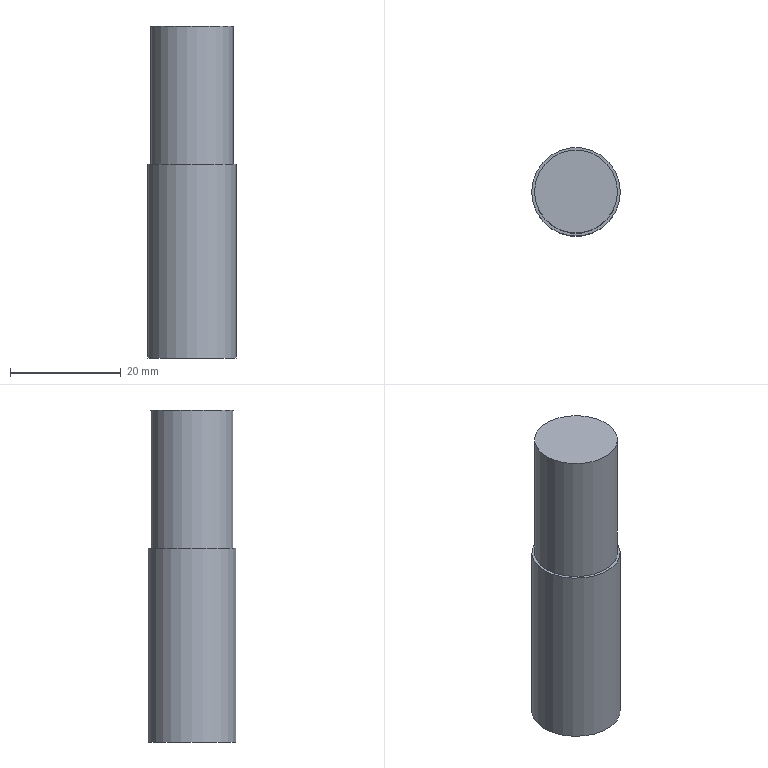Part | NX | features solid 2 | 1 solid | 9 faces | box 16 x 16 x 60 mm | volume 7277 mm3 | plane 5 | cylinder 4 | commonest cylinder face diameters 8 x1 10 x1 15 x1 16 x1
STEP:
#1=CARTESIAN_POINT('',(-635.,-700.,-65.));
#2=VERTEX_POINT('',#1);
#3=CARTESIAN_POINT('',(-630.,-700.,-65.));
#4=DIRECTION('',(0.,0.,-1.));
#5=DIRECTION('',(-1.,0.,0.));
#6=AXIS2_PLACEMENT_3D('',#3,#4,#5);
#7=CIRCLE('',#6,5.);
#8=EDGE_CURVE('',#2,#2,#7,.T.);
#9=ORIENTED_EDGE('',*,*,#8,.F.);
#10=EDGE_LOOP('',(#9));
#11=FACE_BOUND('',#10,.T.);
#12=CARTESIAN_POINT('',(-635.,-700.,-115.));
#13=VERTEX_POINT('',#12);
#14=CARTESIAN_POINT('',(-630.,-700.,-115.));
#15=DIRECTION('',(0.,0.,-1.));
#16=DIRECTION('',(-1.,0.,0.));
#17=AXIS2_PLACEMENT_3D('',#14,#15,#16);
#18=CIRCLE('',#17,5.);
#19=EDGE_CURVE('',#13,#13,#18,.T.);
#20=ORIENTED_EDGE('',*,*,#19,.T.);
#21=EDGE_LOOP('',(#20));
#22=FACE_BOUND('',#21,.T.);
#23=CARTESIAN_POINT('',(-630.,-700.,-65.));
#24=DIRECTION('',(0.,0.,-1.));
#25=DIRECTION('',(-1.,0.,0.));
#26=AXIS2_PLACEMENT_3D('',#23,#24,#25);
#27=CYLINDRICAL_SURFACE('',#26,5.);
#28=ADVANCED_FACE('',(#11,#22),#27,.F.);
#29=ORIENTED_EDGE('',*,*,#8,.T.);
#30=EDGE_LOOP('',(#29));
#31=FACE_BOUND('',#30,.T.);
#32=CARTESIAN_POINT('',(-630.,-700.,-65.));
#33=DIRECTION('',(0.,0.,-1.));
#34=DIRECTION('',(-1.,0.,0.));
#35=AXIS2_PLACEMENT_3D('',#32,#33,#34);
#36=PLANE('',#35);
#37=ADVANCED_FACE('',(#31),#36,.T.);
#38=CARTESIAN_POINT('',(-634.,-700.,-115.));
#39=VERTEX_POINT('',#38);
#40=CARTESIAN_POINT('',(-630.,-700.,-115.));
#41=DIRECTION('',(0.,0.,-1.));
#42=DIRECTION('',(-1.,0.,0.));
#43=AXIS2_PLACEMENT_3D('',#40,#41,#42);
#44=CIRCLE('',#43,4.);
#45=EDGE_CURVE('',#39,#39,#44,.T.);
#46=ORIENTED_EDGE('',*,*,#45,.T.);
#47=EDGE_LOOP('',(#46));
#48=FACE_BOUND('',#47,.T.);
#49=ORIENTED_EDGE('',*,*,#19,.F.);
#50=EDGE_LOOP('',(#49));
#51=FACE_BOUND('',#50,.T.);
#52=CARTESIAN_POINT('',(-630.,-700.,-115.));
#53=DIRECTION('',(0.,0.,-1.));
#54=DIRECTION('',(-1.,0.,0.));
#55=AXIS2_PLACEMENT_3D('',#52,#53,#54);
#56=PLANE('',#55);
#57=ADVANCED_FACE('',(#48,#51),#56,.F.);
#58=CARTESIAN_POINT('',(-634.,-700.,-120.));
#59=VERTEX_POINT('',#58);
#60=CARTESIAN_POINT('',(-630.,-700.,-120.));
#61=DIRECTION('',(0.,0.,-1.));
#62=DIRECTION('',(-1.,0.,0.));
#63=AXIS2_PLACEMENT_3D('',#60,#61,#62);
#64=CIRCLE('',#63,4.);
#65=EDGE_CURVE('',#59,#59,#64,.T.);
#66=ORIENTED_EDGE('',*,*,#65,.T.);
#67=EDGE_LOOP('',(#66));
#68=FACE_BOUND('',#67,.T.);
#69=ORIENTED_EDGE('',*,*,#45,.F.);
#70=EDGE_LOOP('',(#69));
#71=FACE_BOUND('',#70,.T.);
#72=CARTESIAN_POINT('',(-630.,-700.,-110.));
#73=DIRECTION('',(0.,0.,-1.));
#74=DIRECTION('',(-1.,0.,0.));
#75=AXIS2_PLACEMENT_3D('',#72,#73,#74);
#76=CYLINDRICAL_SURFACE('',#75,4.);
#77=ADVANCED_FACE('',(#68,#71),#76,.F.);
#78=CARTESIAN_POINT('',(-637.5,-700.,-60.));
#79=VERTEX_POINT('',#78);
#80=CARTESIAN_POINT('',(-630.,-700.,-60.));
#81=DIRECTION('',(0.,0.,-1.));
#82=DIRECTION('',(-1.,0.,0.));
#83=AXIS2_PLACEMENT_3D('',#80,#81,#82);
#84=CIRCLE('',#83,7.5);
#85=EDGE_CURVE('',#79,#79,#84,.T.);
#86=ORIENTED_EDGE('',*,*,#85,.T.);
#87=EDGE_LOOP('',(#86));
#88=FACE_BOUND('',#87,.T.);
#89=CARTESIAN_POINT('',(-637.5,-700.,-85.));
#90=VERTEX_POINT('',#89);
#91=CARTESIAN_POINT('',(-630.,-700.,-85.));
#92=DIRECTION('',(0.,0.,-1.));
#93=DIRECTION('',(-1.,0.,0.));
#94=AXIS2_PLACEMENT_3D('',#91,#92,#93);
#95=CIRCLE('',#94,7.5);
#96=EDGE_CURVE('',#90,#90,#95,.T.);
#97=ORIENTED_EDGE('',*,*,#96,.F.);
#98=EDGE_LOOP('',(#97));
#99=FACE_BOUND('',#98,.T.);
#100=CARTESIAN_POINT('',(-630.,-700.,-60.));
#101=DIRECTION('',(0.,0.,-1.));
#102=DIRECTION('',(-1.,0.,0.));
#103=AXIS2_PLACEMENT_3D('',#100,#101,#102);
#104=CYLINDRICAL_SURFACE('',#103,7.5);
#105=ADVANCED_FACE('',(#88,#99),#104,.T.);
#106=ORIENTED_EDGE('',*,*,#85,.F.);
#107=EDGE_LOOP('',(#106));
#108=FACE_BOUND('',#107,.T.);
#109=CARTESIAN_POINT('',(-630.,-700.,-60.));
#110=DIRECTION('',(0.,0.,-1.));
#111=DIRECTION('',(-1.,0.,0.));
#112=AXIS2_PLACEMENT_3D('',#109,#110,#111);
#113=PLANE('',#112);
#114=ADVANCED_FACE('',(#108),#113,.F.);
#115=CARTESIAN_POINT('',(-638.,-700.,-85.));
#116=VERTEX_POINT('',#115);
#117=CARTESIAN_POINT('',(-630.,-700.,-85.));
#118=DIRECTION('',(0.,0.,-1.));
#119=DIRECTION('',(-1.,0.,0.));
#120=AXIS2_PLACEMENT_3D('',#117,#118,#119);
#121=CIRCLE('',#120,8.);
#122=EDGE_CURVE('',#116,#116,#121,.T.);
#123=ORIENTED_EDGE('',*,*,#122,.T.);
#124=EDGE_LOOP('',(#123));
#125=FACE_BOUND('',#124,.T.);
#126=CARTESIAN_POINT('',(-638.,-700.,-120.));
#127=VERTEX_POINT('',#126);
#128=CARTESIAN_POINT('',(-630.,-700.,-120.));
#129=DIRECTION('',(0.,0.,-1.));
#130=DIRECTION('',(-1.,0.,0.));
#131=AXIS2_PLACEMENT_3D('',#128,#129,#130);
#132=CIRCLE('',#131,8.);
#133=EDGE_CURVE('',#127,#127,#132,.T.);
#134=ORIENTED_EDGE('',*,*,#133,.F.);
#135=EDGE_LOOP('',(#134));
#136=FACE_BOUND('',#135,.T.);
#137=CARTESIAN_POINT('',(-630.,-700.,-85.));
#138=DIRECTION('',(0.,0.,-1.));
#139=DIRECTION('',(-1.,0.,0.));
#140=AXIS2_PLACEMENT_3D('',#137,#138,#139);
#141=CYLINDRICAL_SURFACE('',#140,8.);
#142=ADVANCED_FACE('',(#125,#136),#141,.T.);
#143=ORIENTED_EDGE('',*,*,#96,.T.);
#144=EDGE_LOOP('',(#143));
#145=FACE_BOUND('',#144,.T.);
#146=ORIENTED_EDGE('',*,*,#122,.F.);
#147=EDGE_LOOP('',(#146));
#148=FACE_BOUND('',#147,.T.);
#149=CARTESIAN_POINT('',(-630.,-700.,-85.));
#150=DIRECTION('',(0.,0.,-1.));
#151=DIRECTION('',(-1.,0.,0.));
#152=AXIS2_PLACEMENT_3D('',#149,#150,#151);
#153=PLANE('',#152);
#154=ADVANCED_FACE('',(#145,#148),#153,.F.);
#155=ORIENTED_EDGE('',*,*,#65,.F.);
#156=EDGE_LOOP('',(#155));
#157=FACE_BOUND('',#156,.T.);
#158=ORIENTED_EDGE('',*,*,#133,.T.);
#159=EDGE_LOOP('',(#158));
#160=FACE_BOUND('',#159,.T.);
#161=CARTESIAN_POINT('',(-630.,-700.,-120.));
#162=DIRECTION('',(0.,0.,-1.));
#163=DIRECTION('',(-1.,0.,0.));
#164=AXIS2_PLACEMENT_3D('',#161,#162,#163);
#165=PLANE('',#164);
#166=ADVANCED_FACE('',(#157,#160),#165,.T.);
#167=CLOSED_SHELL('',(#28,#37,#57,#77,#105,#114,#142,#154,#166));
#168=MANIFOLD_SOLID_BREP('',#167);
#169=(LENGTH_UNIT()NAMED_UNIT(*)SI_UNIT(.MILLI.,.METRE.));
#170=UNCERTAINTY_MEASURE_WITH_UNIT(LENGTH_MEASURE(0.00001),#169,'','');
#171=(NAMED_UNIT(*)PLANE_ANGLE_UNIT()SI_UNIT($,.RADIAN.));
#172=(NAMED_UNIT(*)SI_UNIT($,.STERADIAN.)SOLID_ANGLE_UNIT());
#173=(GEOMETRIC_REPRESENTATION_CONTEXT(3)GLOBAL_UNCERTAINTY_ASSIGNED_CONTEXT((#170))GLOBAL_UNIT_ASSIGNED_CONTEXT((#169,#171,#172))REPRESENTATION_CONTEXT('',''));
#174=ADVANCED_BREP_SHAPE_REPRESENTATION('',(#168),#173);